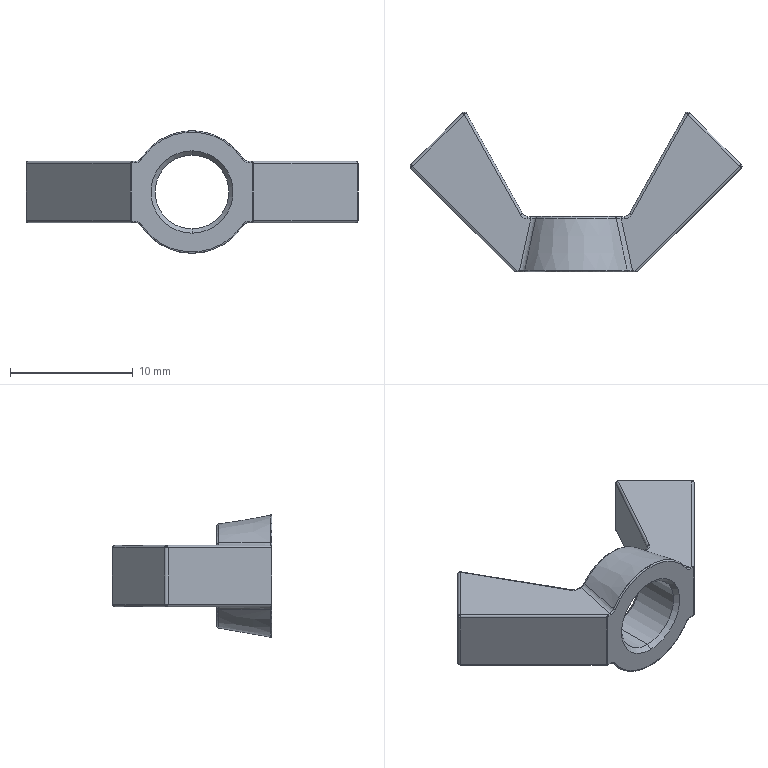Part | SolidWorks | features BaseBody 1 | 1 solid | 92 faces | box 27 x 13 x 9.962 mm | volume 713.416 mm3 | spline 42 | cylinder 31 | plane 12 | cone 7 | commonest cylinder face diameters 0.4 x21 0.2 x6 1 x2 6 x2